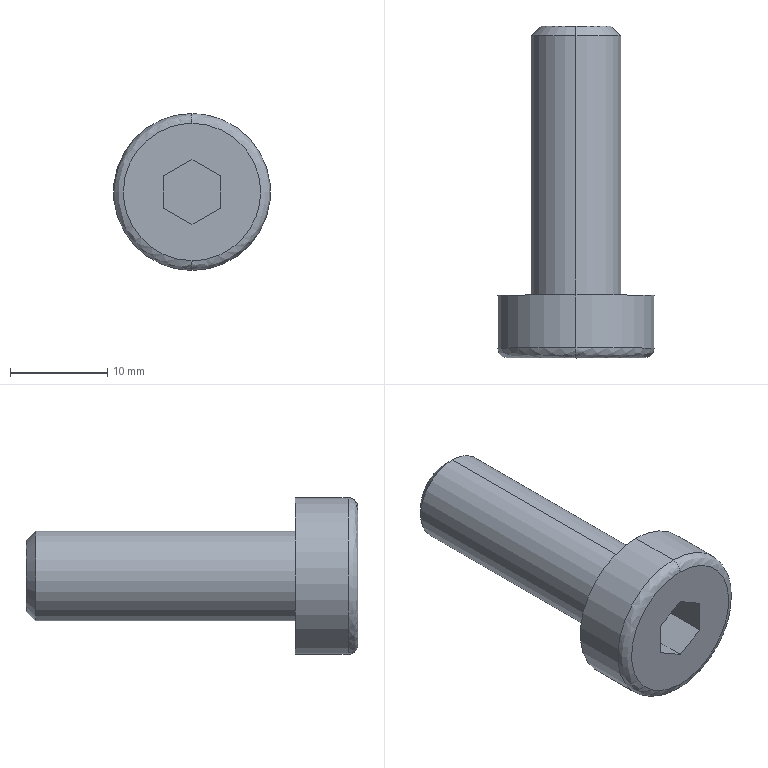Part | SolidWorks | features BaseBody 1 | 1 solid | 18 faces | box 16.154 x 34.154 x 16.154 mm | volume 3001 mm3 | plane 10 | cylinder 4 | spline 2 | cone 2 | commonest cylinder face diameters 9.231 x2 16.154 x2
STEP:
#1=CARTESIAN_POINT('',(57.247,339.356,115.769));
#2=VERTEX_POINT('',#1);
#3=CARTESIAN_POINT('',(57.247,339.356,99.615));
#4=VERTEX_POINT('',#3);
#5=CARTESIAN_POINT('',(57.247,339.356,107.692));
#6=DIRECTION('',(0.,1.,0.));
#7=DIRECTION('',(0.,0.,-1.));
#8=AXIS2_PLACEMENT_3D('',#5,#6,#7);
#9=CIRCLE('',#8,8.077);
#10=EDGE_CURVE('',#2,#4,#9,.T.);
#11=ORIENTED_EDGE('',*,*,#10,.F.);
#12=CARTESIAN_POINT('',(57.247,338.346,114.76));
#13=VERTEX_POINT('',#12);
#14=CARTESIAN_POINT('',(57.247,339.356,114.76));
#15=DIRECTION('',(1.,0.,0.));
#16=DIRECTION('',(0.,0.,1.));
#17=AXIS2_PLACEMENT_3D('',#14,#15,#16);
#18=CIRCLE('',#17,1.01);
#19=EDGE_CURVE('',#2,#13,#18,.T.);
#20=ORIENTED_EDGE('',*,*,#19,.T.);
#21=CARTESIAN_POINT('',(57.247,338.346,100.625));
#22=VERTEX_POINT('',#21);
#23=CARTESIAN_POINT('',(57.247,338.346,114.76));
#24=CARTESIAN_POINT('',(71.381,338.346,114.76));
#25=CARTESIAN_POINT('',(71.381,338.346,100.625));
#26=CARTESIAN_POINT('',(57.247,338.346,100.625));
#27=(BOUNDED_CURVE()B_SPLINE_CURVE(3,(#23,#24,#25,#26),.UNSPECIFIED.,.F.,.F.)B_SPLINE_CURVE_WITH_KNOTS((4,4),(0.,1.),.UNSPECIFIED.)CURVE()GEOMETRIC_REPRESENTATION_ITEM()RATIONAL_B_SPLINE_CURVE((1.,0.3333,0.3333,1.))REPRESENTATION_ITEM(''));
#28=EDGE_CURVE('',#13,#22,#27,.T.);
#29=ORIENTED_EDGE('',*,*,#28,.T.);
#30=CARTESIAN_POINT('',(57.247,339.356,100.625));
#31=DIRECTION('',(-1.,0.,0.));
#32=DIRECTION('',(0.,0.,-1.));
#33=AXIS2_PLACEMENT_3D('',#30,#31,#32);
#34=CIRCLE('',#33,1.01);
#35=EDGE_CURVE('',#4,#22,#34,.T.);
#36=ORIENTED_EDGE('',*,*,#35,.F.);
#37=EDGE_LOOP('',(#11,#20,#29,#36));
#38=FACE_OUTER_BOUND('',#37,.T.);
#39=CARTESIAN_POINT('',(57.247,339.356,115.769));
#40=CARTESIAN_POINT('',(73.4,339.356,115.769));
#41=CARTESIAN_POINT('',(73.4,339.356,99.615));
#42=CARTESIAN_POINT('',(57.247,339.356,99.615));
#43=CARTESIAN_POINT('',(57.247,338.764,115.769));
#44=CARTESIAN_POINT('',(73.4,338.764,115.769));
#45=CARTESIAN_POINT('',(73.4,338.764,99.615));
#46=CARTESIAN_POINT('',(57.247,338.764,99.615));
#47=CARTESIAN_POINT('',(57.247,338.346,115.351));
#48=CARTESIAN_POINT('',(72.564,338.346,115.351));
#49=CARTESIAN_POINT('',(72.564,338.346,100.034));
#50=CARTESIAN_POINT('',(57.247,338.346,100.034));
#51=CARTESIAN_POINT('',(57.247,338.346,114.76));
#52=CARTESIAN_POINT('',(71.381,338.346,114.76));
#53=CARTESIAN_POINT('',(71.381,338.346,100.625));
#54=CARTESIAN_POINT('',(57.247,338.346,100.625));
#55=(BOUNDED_SURFACE()B_SPLINE_SURFACE(3,3,((#39,#40,#41,#42),(#43,#44,#45,#46),(#47,#48,#49,#50),(#51,#52,#53,#54)),.UNSPECIFIED.,.F.,.F.,.T.)B_SPLINE_SURFACE_WITH_KNOTS((4,4),(4,4),(0.,1.),(0.,1.),.UNSPECIFIED.)GEOMETRIC_REPRESENTATION_ITEM()RATIONAL_B_SPLINE_SURFACE(((1.,0.3333,0.3333,1.),(0.8047,0.2682,0.2682,0.8047),(0.8047,0.2682,0.2682,0.8047),(1.,0.3333,0.3333,1.)))REPRESENTATION_ITEM('')SURFACE());
#56=ADVANCED_FACE('',(#38),#55,.T.);
#57=CARTESIAN_POINT('',(57.247,371.509,103.077));
#58=VERTEX_POINT('',#57);
#59=CARTESIAN_POINT('',(57.247,371.509,112.308));
#60=VERTEX_POINT('',#59);
#61=CARTESIAN_POINT('',(57.247,371.509,107.692));
#62=DIRECTION('',(0.,-1.,0.));
#63=DIRECTION('',(0.,0.,-1.));
#64=AXIS2_PLACEMENT_3D('',#61,#62,#63);
#65=CIRCLE('',#64,4.615);
#66=EDGE_CURVE('',#58,#60,#65,.T.);
#67=ORIENTED_EDGE('',*,*,#66,.T.);
#68=CARTESIAN_POINT('',(57.247,344.808,112.308));
#69=VERTEX_POINT('',#68);
#70=CARTESIAN_POINT('',(57.247,372.5,112.308));
#71=DIRECTION('',(0.,-1.,0.));
#72=VECTOR('',#71,1000.);
#73=LINE('',#70,#72);
#74=EDGE_CURVE('',#60,#69,#73,.T.);
#75=ORIENTED_EDGE('',*,*,#74,.T.);
#76=CARTESIAN_POINT('',(57.247,344.808,103.077));
#77=VERTEX_POINT('',#76);
#78=CARTESIAN_POINT('',(57.247,344.808,107.692));
#79=DIRECTION('',(0.,1.,0.));
#80=DIRECTION('',(0.,0.,-1.));
#81=AXIS2_PLACEMENT_3D('',#78,#79,#80);
#82=CIRCLE('',#81,4.615);
#83=EDGE_CURVE('',#69,#77,#82,.T.);
#84=ORIENTED_EDGE('',*,*,#83,.T.);
#85=CARTESIAN_POINT('',(57.247,372.5,103.077));
#86=DIRECTION('',(0.,-1.,0.));
#87=VECTOR('',#86,1000.);
#88=LINE('',#85,#87);
#89=EDGE_CURVE('',#58,#77,#88,.T.);
#90=ORIENTED_EDGE('',*,*,#89,.F.);
#91=EDGE_LOOP('',(#67,#75,#84,#90));
#92=FACE_OUTER_BOUND('',#91,.T.);
#93=CARTESIAN_POINT('',(57.247,372.5,107.692));
#94=DIRECTION('',(0.,-1.,0.));
#95=DIRECTION('',(0.,0.,-1.));
#96=AXIS2_PLACEMENT_3D('',#93,#94,#95);
#97=CYLINDRICAL_SURFACE('',#96,4.615);
#98=ADVANCED_FACE('',(#92),#97,.T.);
#99=CARTESIAN_POINT('',(57.247,372.5,104.068));
#100=VERTEX_POINT('',#99);
#101=CARTESIAN_POINT('',(57.247,372.5,111.317));
#102=VERTEX_POINT('',#101);
#103=CARTESIAN_POINT('',(57.247,372.5,107.692));
#104=DIRECTION('',(0.,-1.,0.));
#105=DIRECTION('',(0.,0.,-1.));
#106=AXIS2_PLACEMENT_3D('',#103,#104,#105);
#107=CIRCLE('',#106,3.624);
#108=EDGE_CURVE('',#100,#102,#107,.T.);
#109=ORIENTED_EDGE('',*,*,#108,.T.);
#110=CARTESIAN_POINT('',(57.247,371.509,112.308));
#111=DIRECTION('',(0.,-0.7071,0.7071));
#112=VECTOR('',#111,1000.);
#113=LINE('',#110,#112);
#114=EDGE_CURVE('',#102,#60,#113,.T.);
#115=ORIENTED_EDGE('',*,*,#114,.T.);
#116=ORIENTED_EDGE('',*,*,#66,.F.);
#117=CARTESIAN_POINT('',(57.247,371.509,103.077));
#118=DIRECTION('',(0.,-0.7071,-0.7071));
#119=VECTOR('',#118,1000.);
#120=LINE('',#117,#119);
#121=EDGE_CURVE('',#100,#58,#120,.T.);
#122=ORIENTED_EDGE('',*,*,#121,.F.);
#123=EDGE_LOOP('',(#109,#115,#116,#122));
#124=FACE_OUTER_BOUND('',#123,.T.);
#125=CARTESIAN_POINT('',(57.247,371.509,107.692));
#126=DIRECTION('',(0.,-1.,0.));
#127=DIRECTION('',(0.,0.,-1.));
#128=AXIS2_PLACEMENT_3D('',#125,#126,#127);
#129=CONICAL_SURFACE('',#128,4.615,0.7854);
#130=ADVANCED_FACE('',(#124),#129,.T.);
#131=CARTESIAN_POINT('',(57.247,344.808,99.615));
#132=VERTEX_POINT('',#131);
#133=CARTESIAN_POINT('',(57.247,344.808,115.769));
#134=VERTEX_POINT('',#133);
#135=CARTESIAN_POINT('',(57.247,344.808,107.692));
#136=DIRECTION('',(0.,-1.,0.));
#137=DIRECTION('',(0.,0.,-1.));
#138=AXIS2_PLACEMENT_3D('',#135,#136,#137);
#139=CIRCLE('',#138,8.077);
#140=EDGE_CURVE('',#132,#134,#139,.T.);
#141=ORIENTED_EDGE('',*,*,#140,.T.);
#142=CARTESIAN_POINT('',(57.247,372.5,115.769));
#143=DIRECTION('',(0.,-1.,0.));
#144=VECTOR('',#143,1000.);
#145=LINE('',#142,#144);
#146=EDGE_CURVE('',#134,#2,#145,.T.);
#147=ORIENTED_EDGE('',*,*,#146,.T.);
#148=ORIENTED_EDGE('',*,*,#10,.T.);
#149=CARTESIAN_POINT('',(57.247,372.5,99.615));
#150=DIRECTION('',(0.,-1.,0.));
#151=VECTOR('',#150,1000.);
#152=LINE('',#149,#151);
#153=EDGE_CURVE('',#132,#4,#152,.T.);
#154=ORIENTED_EDGE('',*,*,#153,.F.);
#155=EDGE_LOOP('',(#141,#147,#148,#154));
#156=FACE_OUTER_BOUND('',#155,.T.);
#157=CARTESIAN_POINT('',(57.247,372.5,107.692));
#158=DIRECTION('',(0.,-1.,0.));
#159=DIRECTION('',(0.,0.,-1.));
#160=AXIS2_PLACEMENT_3D('',#157,#158,#159);
#161=CYLINDRICAL_SURFACE('',#160,8.077);
#162=ADVANCED_FACE('',(#156),#161,.T.);
#163=ORIENTED_EDGE('',*,*,#74,.F.);
#164=CARTESIAN_POINT('',(57.247,371.509,107.692));
#165=DIRECTION('',(0.,-1.,0.));
#166=DIRECTION('',(0.,0.,-1.));
#167=AXIS2_PLACEMENT_3D('',#164,#165,#166);
#168=CIRCLE('',#167,4.615);
#169=EDGE_CURVE('',#60,#58,#168,.T.);
#170=ORIENTED_EDGE('',*,*,#169,.T.);
#171=ORIENTED_EDGE('',*,*,#89,.T.);
#172=CARTESIAN_POINT('',(57.247,344.808,107.692));
#173=DIRECTION('',(0.,1.,0.));
#174=DIRECTION('',(0.,0.,-1.));
#175=AXIS2_PLACEMENT_3D('',#172,#173,#174);
#176=CIRCLE('',#175,4.615);
#177=EDGE_CURVE('',#77,#69,#176,.T.);
#178=ORIENTED_EDGE('',*,*,#177,.T.);
#179=EDGE_LOOP('',(#163,#170,#171,#178));
#180=FACE_OUTER_BOUND('',#179,.T.);
#181=CARTESIAN_POINT('',(57.247,372.5,107.692));
#182=DIRECTION('',(0.,-1.,0.));
#183=DIRECTION('',(0.,0.,-1.));
#184=AXIS2_PLACEMENT_3D('',#181,#182,#183);
#185=CYLINDRICAL_SURFACE('',#184,4.615);
#186=ADVANCED_FACE('',(#180),#185,.T.);
#187=ORIENTED_EDGE('',*,*,#177,.F.);
#188=ORIENTED_EDGE('',*,*,#83,.F.);
#189=EDGE_LOOP('',(#187,#188));
#190=FACE_BOUND('',#189,.T.);
#191=ORIENTED_EDGE('',*,*,#140,.F.);
#192=CARTESIAN_POINT('',(57.247,344.808,107.692));
#193=DIRECTION('',(0.,-1.,0.));
#194=DIRECTION('',(0.,0.,-1.));
#195=AXIS2_PLACEMENT_3D('',#192,#193,#194);
#196=CIRCLE('',#195,8.077);
#197=EDGE_CURVE('',#134,#132,#196,.T.);
#198=ORIENTED_EDGE('',*,*,#197,.F.);
#199=EDGE_LOOP('',(#191,#198));
#200=FACE_OUTER_BOUND('',#199,.T.);
#201=CARTESIAN_POINT('',(57.247,344.808,99.615));
#202=DIRECTION('',(0.,-1.,0.));
#203=DIRECTION('',(0.,0.,-1.));
#204=AXIS2_PLACEMENT_3D('',#201,#202,#203);
#205=PLANE('',#204);
#206=ADVANCED_FACE('',(#190,#200),#205,.F.);
#207=ORIENTED_EDGE('',*,*,#114,.F.);
#208=CARTESIAN_POINT('',(57.247,372.5,107.692));
#209=DIRECTION('',(0.,-1.,0.));
#210=DIRECTION('',(0.,0.,-1.));
#211=AXIS2_PLACEMENT_3D('',#208,#209,#210);
#212=CIRCLE('',#211,3.624);
#213=EDGE_CURVE('',#102,#100,#212,.T.);
#214=ORIENTED_EDGE('',*,*,#213,.T.);
#215=ORIENTED_EDGE('',*,*,#121,.T.);
#216=ORIENTED_EDGE('',*,*,#169,.F.);
#217=EDGE_LOOP('',(#207,#214,#215,#216));
#218=FACE_OUTER_BOUND('',#217,.T.);
#219=CARTESIAN_POINT('',(57.247,371.509,107.692));
#220=DIRECTION('',(0.,-1.,0.));
#221=DIRECTION('',(0.,0.,-1.));
#222=AXIS2_PLACEMENT_3D('',#219,#220,#221);
#223=CONICAL_SURFACE('',#222,4.615,0.7854);
#224=ADVANCED_FACE('',(#218),#223,.T.);
#225=ORIENTED_EDGE('',*,*,#146,.F.);
#226=ORIENTED_EDGE('',*,*,#197,.T.);
#227=ORIENTED_EDGE('',*,*,#153,.T.);
#228=CARTESIAN_POINT('',(57.247,339.356,107.692));
#229=DIRECTION('',(0.,1.,0.));
#230=DIRECTION('',(0.,0.,-1.));
#231=AXIS2_PLACEMENT_3D('',#228,#229,#230);
#232=CIRCLE('',#231,8.077);
#233=EDGE_CURVE('',#4,#2,#232,.T.);
#234=ORIENTED_EDGE('',*,*,#233,.T.);
#235=EDGE_LOOP('',(#225,#226,#227,#234));
#236=FACE_OUTER_BOUND('',#235,.T.);
#237=CARTESIAN_POINT('',(57.247,372.5,107.692));
#238=DIRECTION('',(0.,-1.,0.));
#239=DIRECTION('',(0.,0.,-1.));
#240=AXIS2_PLACEMENT_3D('',#237,#238,#239);
#241=CYLINDRICAL_SURFACE('',#240,8.077);
#242=ADVANCED_FACE('',(#236),#241,.T.);
#243=ORIENTED_EDGE('',*,*,#108,.F.);
#244=ORIENTED_EDGE('',*,*,#213,.F.);
#245=EDGE_LOOP('',(#243,#244));
#246=FACE_OUTER_BOUND('',#245,.T.);
#247=CARTESIAN_POINT('',(57.247,372.5,104.068));
#248=DIRECTION('',(0.,-1.,0.));
#249=DIRECTION('',(0.,0.,-1.));
#250=AXIS2_PLACEMENT_3D('',#247,#248,#249);
#251=PLANE('',#250);
#252=ADVANCED_FACE('',(#246),#251,.F.);
#253=ORIENTED_EDGE('',*,*,#19,.F.);
#254=ORIENTED_EDGE('',*,*,#233,.F.);
#255=ORIENTED_EDGE('',*,*,#35,.T.);
#256=CARTESIAN_POINT('',(50.179,338.346,107.692));
#257=VERTEX_POINT('',#256);
#258=CARTESIAN_POINT('',(57.247,338.346,100.625));
#259=CARTESIAN_POINT('',(53.107,338.346,100.625));
#260=CARTESIAN_POINT('',(50.179,338.346,103.552));
#261=CARTESIAN_POINT('',(50.179,338.346,107.692));
#262=(BOUNDED_CURVE()B_SPLINE_CURVE(3,(#258,#259,#260,#261),.UNSPECIFIED.,.F.,.F.)B_SPLINE_CURVE_WITH_KNOTS((4,4),(0.,1.),.UNSPECIFIED.)CURVE()GEOMETRIC_REPRESENTATION_ITEM()RATIONAL_B_SPLINE_CURVE((1.,0.8047,0.8047,1.))REPRESENTATION_ITEM(''));
#263=EDGE_CURVE('',#22,#257,#262,.T.);
#264=ORIENTED_EDGE('',*,*,#263,.T.);
#265=CARTESIAN_POINT('',(50.179,338.346,107.692));
#266=CARTESIAN_POINT('',(50.179,338.346,111.832));
#267=CARTESIAN_POINT('',(53.107,338.346,114.76));
#268=CARTESIAN_POINT('',(57.247,338.346,114.76));
#269=(BOUNDED_CURVE()B_SPLINE_CURVE(3,(#265,#266,#267,#268),.UNSPECIFIED.,.F.,.F.)B_SPLINE_CURVE_WITH_KNOTS((4,4),(0.,1.),.UNSPECIFIED.)CURVE()GEOMETRIC_REPRESENTATION_ITEM()RATIONAL_B_SPLINE_CURVE((1.,0.8047,0.8047,1.))REPRESENTATION_ITEM(''));
#270=EDGE_CURVE('',#257,#13,#269,.T.);
#271=ORIENTED_EDGE('',*,*,#270,.T.);
#272=EDGE_LOOP('',(#253,#254,#255,#264,#271));
#273=FACE_OUTER_BOUND('',#272,.T.);
#274=CARTESIAN_POINT('',(57.247,339.356,99.615));
#275=CARTESIAN_POINT('',(41.093,339.356,99.615));
#276=CARTESIAN_POINT('',(41.093,339.356,115.769));
#277=CARTESIAN_POINT('',(57.247,339.356,115.769));
#278=CARTESIAN_POINT('',(57.247,338.764,99.615));
#279=CARTESIAN_POINT('',(41.093,338.764,99.615));
#280=CARTESIAN_POINT('',(41.093,338.764,115.769));
#281=CARTESIAN_POINT('',(57.247,338.764,115.769));
#282=CARTESIAN_POINT('',(57.247,338.346,100.034));
#283=CARTESIAN_POINT('',(41.929,338.346,100.034));
#284=CARTESIAN_POINT('',(41.929,338.346,115.351));
#285=CARTESIAN_POINT('',(57.247,338.346,115.351));
#286=CARTESIAN_POINT('',(57.247,338.346,100.625));
#287=CARTESIAN_POINT('',(43.112,338.346,100.625));
#288=CARTESIAN_POINT('',(43.112,338.346,114.76));
#289=CARTESIAN_POINT('',(57.247,338.346,114.76));
#290=(BOUNDED_SURFACE()B_SPLINE_SURFACE(3,3,((#274,#275,#276,#277),(#278,#279,#280,#281),(#282,#283,#284,#285),(#286,#287,#288,#289)),.UNSPECIFIED.,.F.,.F.,.F.)B_SPLINE_SURFACE_WITH_KNOTS((4,4),(4,4),(0.,1.),(0.,1.),.UNSPECIFIED.)GEOMETRIC_REPRESENTATION_ITEM()RATIONAL_B_SPLINE_SURFACE(((1.,0.3333,0.3333,1.),(0.8047,0.2682,0.2682,0.8047),(0.8047,0.2682,0.2682,0.8047),(1.,0.3333,0.3333,1.)))REPRESENTATION_ITEM('')SURFACE());
#291=ADVANCED_FACE('',(#273),#290,.T.);
#292=CARTESIAN_POINT('',(57.247,338.346,104.361));
#293=VERTEX_POINT('',#292);
#294=CARTESIAN_POINT('',(60.131,338.346,106.027));
#295=VERTEX_POINT('',#294);
#296=CARTESIAN_POINT('',(57.247,338.346,104.361));
#297=DIRECTION('',(0.866,0.,0.5));
#298=VECTOR('',#297,1000.);
#299=LINE('',#296,#298);
#300=EDGE_CURVE('',#293,#295,#299,.T.);
#301=ORIENTED_EDGE('',*,*,#300,.F.);
#302=CARTESIAN_POINT('',(54.362,338.346,106.027));
#303=VERTEX_POINT('',#302);
#304=CARTESIAN_POINT('',(54.362,338.346,106.027));
#305=DIRECTION('',(0.866,0.,-0.5));
#306=VECTOR('',#305,1000.);
#307=LINE('',#304,#306);
#308=EDGE_CURVE('',#303,#293,#307,.T.);
#309=ORIENTED_EDGE('',*,*,#308,.F.);
#310=CARTESIAN_POINT('',(54.362,338.346,109.358));
#311=VERTEX_POINT('',#310);
#312=CARTESIAN_POINT('',(54.362,338.346,107.692));
#313=DIRECTION('',(0.,0.,-1.));
#314=VECTOR('',#313,1000.);
#315=LINE('',#312,#314);
#316=EDGE_CURVE('',#311,#303,#315,.T.);
#317=ORIENTED_EDGE('',*,*,#316,.F.);
#318=CARTESIAN_POINT('',(57.247,338.346,111.023));
#319=VERTEX_POINT('',#318);
#320=CARTESIAN_POINT('',(57.247,338.346,111.023));
#321=DIRECTION('',(-0.866,0.,-0.5));
#322=VECTOR('',#321,1000.);
#323=LINE('',#320,#322);
#324=EDGE_CURVE('',#319,#311,#323,.T.);
#325=ORIENTED_EDGE('',*,*,#324,.F.);
#326=CARTESIAN_POINT('',(60.131,338.346,109.358));
#327=VERTEX_POINT('',#326);
#328=CARTESIAN_POINT('',(60.131,338.346,109.358));
#329=DIRECTION('',(-0.866,0.,0.5));
#330=VECTOR('',#329,1000.);
#331=LINE('',#328,#330);
#332=EDGE_CURVE('',#327,#319,#331,.T.);
#333=ORIENTED_EDGE('',*,*,#332,.F.);
#334=CARTESIAN_POINT('',(60.131,338.346,107.692));
#335=DIRECTION('',(0.,0.,1.));
#336=VECTOR('',#335,1000.);
#337=LINE('',#334,#336);
#338=EDGE_CURVE('',#295,#327,#337,.T.);
#339=ORIENTED_EDGE('',*,*,#338,.F.);
#340=EDGE_LOOP('',(#301,#309,#317,#325,#333,#339));
#341=FACE_BOUND('',#340,.T.);
#342=ORIENTED_EDGE('',*,*,#28,.F.);
#343=ORIENTED_EDGE('',*,*,#270,.F.);
#344=ORIENTED_EDGE('',*,*,#263,.F.);
#345=EDGE_LOOP('',(#342,#343,#344));
#346=FACE_OUTER_BOUND('',#345,.T.);
#347=CARTESIAN_POINT('',(57.247,338.346,107.692));
#348=DIRECTION('',(0.,1.,0.));
#349=DIRECTION('',(0.,0.,1.));
#350=AXIS2_PLACEMENT_3D('',#347,#348,#349);
#351=PLANE('',#350);
#352=ADVANCED_FACE('',(#341,#346),#351,.F.);
#353=CARTESIAN_POINT('',(60.131,343.654,109.358));
#354=VERTEX_POINT('',#353);
#355=CARTESIAN_POINT('',(60.131,343.654,109.358));
#356=DIRECTION('',(0.,1.,0.));
#357=VECTOR('',#356,1000.);
#358=LINE('',#355,#357);
#359=EDGE_CURVE('',#327,#354,#358,.T.);
#360=ORIENTED_EDGE('',*,*,#359,.T.);
#361=CARTESIAN_POINT('',(60.131,343.654,106.027));
#362=VERTEX_POINT('',#361);
#363=CARTESIAN_POINT('',(60.131,343.654,109.358));
#364=DIRECTION('',(0.,0.,-1.));
#365=VECTOR('',#364,1000.);
#366=LINE('',#363,#365);
#367=EDGE_CURVE('',#354,#362,#366,.T.);
#368=ORIENTED_EDGE('',*,*,#367,.T.);
#369=CARTESIAN_POINT('',(60.131,343.654,106.027));
#370=DIRECTION('',(0.,-1.,0.));
#371=VECTOR('',#370,1000.);
#372=LINE('',#369,#371);
#373=EDGE_CURVE('',#362,#295,#372,.T.);
#374=ORIENTED_EDGE('',*,*,#373,.T.);
#375=ORIENTED_EDGE('',*,*,#338,.T.);
#376=EDGE_LOOP('',(#360,#368,#374,#375));
#377=FACE_OUTER_BOUND('',#376,.T.);
#378=CARTESIAN_POINT('',(60.131,343.654,109.358));
#379=DIRECTION('',(-1.,0.,0.));
#380=DIRECTION('',(0.,0.,1.));
#381=AXIS2_PLACEMENT_3D('',#378,#379,#380);
#382=PLANE('',#381);
#383=ADVANCED_FACE('',(#377),#382,.T.);
#384=ORIENTED_EDGE('',*,*,#373,.F.);
#385=CARTESIAN_POINT('',(57.247,343.654,104.361));
#386=VERTEX_POINT('',#385);
#387=CARTESIAN_POINT('',(60.131,343.654,106.027));
#388=DIRECTION('',(-0.866,0.,-0.5));
#389=VECTOR('',#388,1000.);
#390=LINE('',#387,#389);
#391=EDGE_CURVE('',#362,#386,#390,.T.);
#392=ORIENTED_EDGE('',*,*,#391,.T.);
#393=CARTESIAN_POINT('',(57.247,343.654,104.361));
#394=DIRECTION('',(0.,-1.,0.));
#395=VECTOR('',#394,1000.);
#396=LINE('',#393,#395);
#397=EDGE_CURVE('',#386,#293,#396,.T.);
#398=ORIENTED_EDGE('',*,*,#397,.T.);
#399=ORIENTED_EDGE('',*,*,#300,.T.);
#400=EDGE_LOOP('',(#384,#392,#398,#399));
#401=FACE_OUTER_BOUND('',#400,.T.);
#402=CARTESIAN_POINT('',(60.131,343.654,106.027));
#403=DIRECTION('',(-0.5,0.,0.866));
#404=DIRECTION('',(0.866,0.,0.5));
#405=AXIS2_PLACEMENT_3D('',#402,#403,#404);
#406=PLANE('',#405);
#407=ADVANCED_FACE('',(#401),#406,.T.);
#408=ORIENTED_EDGE('',*,*,#397,.F.);
#409=CARTESIAN_POINT('',(54.362,343.654,106.027));
#410=VERTEX_POINT('',#409);
#411=CARTESIAN_POINT('',(57.247,343.654,104.361));
#412=DIRECTION('',(-0.866,0.,0.5));
#413=VECTOR('',#412,1000.);
#414=LINE('',#411,#413);
#415=EDGE_CURVE('',#386,#410,#414,.T.);
#416=ORIENTED_EDGE('',*,*,#415,.T.);
#417=CARTESIAN_POINT('',(54.362,343.654,106.027));
#418=DIRECTION('',(0.,-1.,0.));
#419=VECTOR('',#418,1000.);
#420=LINE('',#417,#419);
#421=EDGE_CURVE('',#410,#303,#420,.T.);
#422=ORIENTED_EDGE('',*,*,#421,.T.);
#423=ORIENTED_EDGE('',*,*,#308,.T.);
#424=EDGE_LOOP('',(#408,#416,#422,#423));
#425=FACE_OUTER_BOUND('',#424,.T.);
#426=CARTESIAN_POINT('',(57.247,343.654,104.361));
#427=DIRECTION('',(0.5,0.,0.866));
#428=DIRECTION('',(0.866,0.,-0.5));
#429=AXIS2_PLACEMENT_3D('',#426,#427,#428);
#430=PLANE('',#429);
#431=ADVANCED_FACE('',(#425),#430,.T.);
#432=ORIENTED_EDGE('',*,*,#421,.F.);
#433=CARTESIAN_POINT('',(54.362,343.654,109.358));
#434=VERTEX_POINT('',#433);
#435=CARTESIAN_POINT('',(54.362,343.654,106.027));
#436=DIRECTION('',(0.,0.,1.));
#437=VECTOR('',#436,1000.);
#438=LINE('',#435,#437);
#439=EDGE_CURVE('',#410,#434,#438,.T.);
#440=ORIENTED_EDGE('',*,*,#439,.T.);
#441=CARTESIAN_POINT('',(54.362,343.654,109.358));
#442=DIRECTION('',(0.,-1.,0.));
#443=VECTOR('',#442,1000.);
#444=LINE('',#441,#443);
#445=EDGE_CURVE('',#434,#311,#444,.T.);
#446=ORIENTED_EDGE('',*,*,#445,.T.);
#447=ORIENTED_EDGE('',*,*,#316,.T.);
#448=EDGE_LOOP('',(#432,#440,#446,#447));
#449=FACE_OUTER_BOUND('',#448,.T.);
#450=CARTESIAN_POINT('',(54.362,343.654,106.027));
#451=DIRECTION('',(1.,0.,0.));
#452=DIRECTION('',(0.,0.,-1.));
#453=AXIS2_PLACEMENT_3D('',#450,#451,#452);
#454=PLANE('',#453);
#455=ADVANCED_FACE('',(#449),#454,.T.);
#456=ORIENTED_EDGE('',*,*,#445,.F.);
#457=CARTESIAN_POINT('',(57.247,343.654,111.023));
#458=VERTEX_POINT('',#457);
#459=CARTESIAN_POINT('',(54.362,343.654,109.358));
#460=DIRECTION('',(0.866,0.,0.5));
#461=VECTOR('',#460,1000.);
#462=LINE('',#459,#461);
#463=EDGE_CURVE('',#434,#458,#462,.T.);
#464=ORIENTED_EDGE('',*,*,#463,.T.);
#465=CARTESIAN_POINT('',(57.247,343.654,111.023));
#466=DIRECTION('',(0.,-1.,0.));
#467=VECTOR('',#466,1000.);
#468=LINE('',#465,#467);
#469=EDGE_CURVE('',#458,#319,#468,.T.);
#470=ORIENTED_EDGE('',*,*,#469,.T.);
#471=ORIENTED_EDGE('',*,*,#324,.T.);
#472=EDGE_LOOP('',(#456,#464,#470,#471));
#473=FACE_OUTER_BOUND('',#472,.T.);
#474=CARTESIAN_POINT('',(54.362,343.654,109.358));
#475=DIRECTION('',(0.5,0.,-0.866));
#476=DIRECTION('',(-0.866,0.,-0.5));
#477=AXIS2_PLACEMENT_3D('',#474,#475,#476);
#478=PLANE('',#477);
#479=ADVANCED_FACE('',(#473),#478,.T.);
#480=ORIENTED_EDGE('',*,*,#469,.F.);
#481=CARTESIAN_POINT('',(57.247,343.654,111.023));
#482=DIRECTION('',(0.866,0.,-0.5));
#483=VECTOR('',#482,1000.);
#484=LINE('',#481,#483);
#485=EDGE_CURVE('',#458,#354,#484,.T.);
#486=ORIENTED_EDGE('',*,*,#485,.T.);
#487=ORIENTED_EDGE('',*,*,#359,.F.);
#488=ORIENTED_EDGE('',*,*,#332,.T.);
#489=EDGE_LOOP('',(#480,#486,#487,#488));
#490=FACE_OUTER_BOUND('',#489,.T.);
#491=CARTESIAN_POINT('',(57.247,343.654,111.023));
#492=DIRECTION('',(-0.5,0.,-0.866));
#493=DIRECTION('',(-0.866,0.,0.5));
#494=AXIS2_PLACEMENT_3D('',#491,#492,#493);
#495=PLANE('',#494);
#496=ADVANCED_FACE('',(#490),#495,.T.);
#497=ORIENTED_EDGE('',*,*,#391,.F.);
#498=ORIENTED_EDGE('',*,*,#367,.F.);
#499=ORIENTED_EDGE('',*,*,#485,.F.);
#500=ORIENTED_EDGE('',*,*,#463,.F.);
#501=ORIENTED_EDGE('',*,*,#439,.F.);
#502=ORIENTED_EDGE('',*,*,#415,.F.);
#503=EDGE_LOOP('',(#497,#498,#499,#500,#501,#502));
#504=FACE_OUTER_BOUND('',#503,.T.);
#505=CARTESIAN_POINT('',(57.247,343.654,107.692));
#506=DIRECTION('',(0.,1.,0.));
#507=DIRECTION('',(0.,0.,1.));
#508=AXIS2_PLACEMENT_3D('',#505,#506,#507);
#509=PLANE('',#508);
#510=ADVANCED_FACE('',(#504),#509,.F.);
#511=CLOSED_SHELL('',(#56,#98,#130,#162,#186,#206,#224,#242,#252,#291,#352,#383,#407,#431,#455,#479,#496,#510));
#512=MANIFOLD_SOLID_BREP('',#511);
#513=CARTESIAN_POINT('',(0.,0.,0.));
#514=DIRECTION('',(0.,0.,1.));
#515=DIRECTION('',(1.,0.,0.));
#516=AXIS2_PLACEMENT_3D('',#513,#514,#515);
#517=(LENGTH_UNIT()NAMED_UNIT(*)SI_UNIT(.MILLI.,.METRE.));
#518=UNCERTAINTY_MEASURE_WITH_UNIT(LENGTH_MEASURE(0.00001),#517,'','');
#519=(NAMED_UNIT(*)PLANE_ANGLE_UNIT()SI_UNIT($,.RADIAN.));
#520=(NAMED_UNIT(*)SI_UNIT($,.STERADIAN.)SOLID_ANGLE_UNIT());
#521=(GEOMETRIC_REPRESENTATION_CONTEXT(3)GLOBAL_UNCERTAINTY_ASSIGNED_CONTEXT((#518))GLOBAL_UNIT_ASSIGNED_CONTEXT((#517,#519,#520))REPRESENTATION_CONTEXT('',''));
#522=ADVANCED_BREP_SHAPE_REPRESENTATION('',(#512,#516),#521);